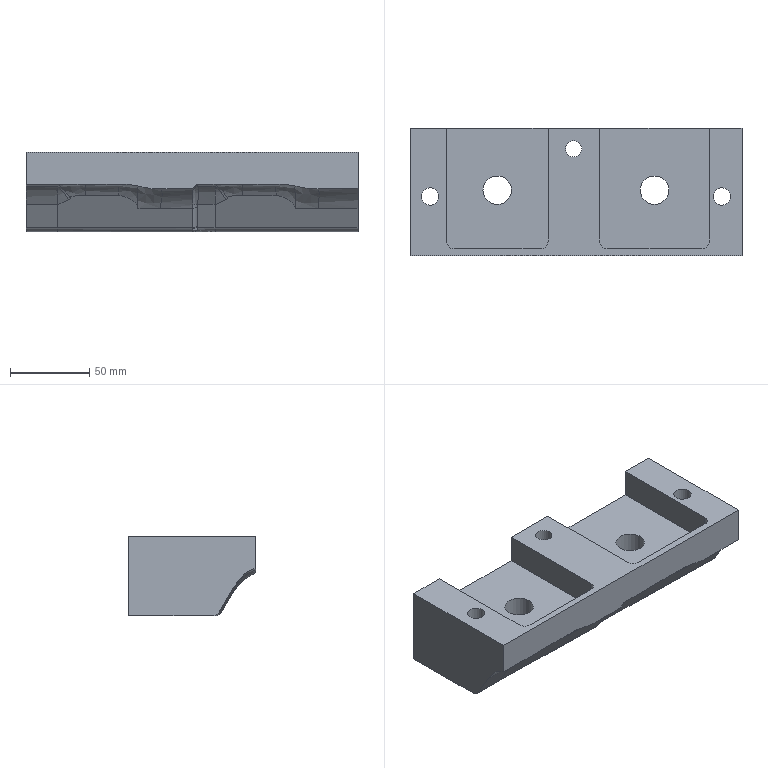Part | NX | features solid 2 | 1 solid | 87 faces | box 209 x 80.002 x 50.25 mm | volume 506272 mm3 | plane 33 | cylinder 27 | spline 27 | commonest cylinder face diameters 6.5 x6 10 x6 6 x4 17 x3 11 x2 18 x2